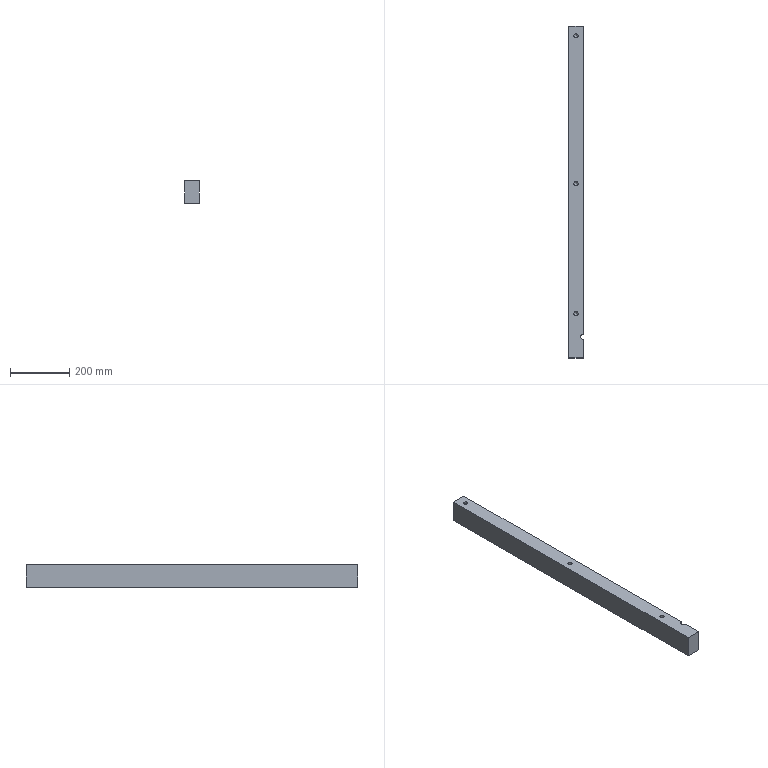Part | NX | features 3 2 | 1 solid | 20 faces | box 50 x 1123 x 75.5 mm | volume 4220069 mm3 | plane 7 | cylinder 7 | cone 6 | commonest cylinder face diameters 14.1 x6 18 x1
STEP:
#1=CARTESIAN_POINT('',(2967.05,-82.5,256.5));
#2=VERTEX_POINT('',#1);
#3=CARTESIAN_POINT('',(2960.,-82.5,256.5));
#4=DIRECTION('',(0.,0.,-1.));
#5=DIRECTION('',(1.,0.,0.));
#6=AXIS2_PLACEMENT_3D('',#3,#4,#5);
#7=CIRCLE('',#6,7.05);
#8=EDGE_CURVE('',#2,#2,#7,.T.);
#9=ORIENTED_EDGE('',*,*,#8,.T.);
#10=EDGE_LOOP('',(#9));
#11=FACE_BOUND('',#10,.T.);
#12=CARTESIAN_POINT('',(2985.,-672.5,256.5));
#13=VERTEX_POINT('',#12);
#14=CARTESIAN_POINT('',(2985.,-609.5,256.5));
#15=VERTEX_POINT('',#14);
#16=CARTESIAN_POINT('',(2985.,193.,256.5));
#17=DIRECTION('',(0.,1.,0.));
#18=VECTOR('',#17,1000.);
#19=LINE('',#16,#18);
#20=EDGE_CURVE('',#13,#15,#19,.T.);
#21=ORIENTED_EDGE('',*,*,#20,.T.);
#22=CARTESIAN_POINT('',(2985.,-591.5,256.5));
#23=VERTEX_POINT('',#22);
#24=CARTESIAN_POINT('',(2985.,-600.5,256.5));
#25=DIRECTION('',(0.,0.,1.));
#26=DIRECTION('',(1.,0.,0.));
#27=AXIS2_PLACEMENT_3D('',#24,#25,#26);
#28=CIRCLE('',#27,9.);
#29=EDGE_CURVE('',#23,#15,#28,.T.);
#30=ORIENTED_EDGE('',*,*,#29,.F.);
#31=CARTESIAN_POINT('',(2985.,450.5,256.5));
#32=VERTEX_POINT('',#31);
#33=CARTESIAN_POINT('',(2985.,193.,256.5));
#34=DIRECTION('',(0.,1.,0.));
#35=VECTOR('',#34,1000.);
#36=LINE('',#33,#35);
#37=EDGE_CURVE('',#23,#32,#36,.T.);
#38=ORIENTED_EDGE('',*,*,#37,.T.);
#39=CARTESIAN_POINT('',(2935.,450.5,256.5));
#40=VERTEX_POINT('',#39);
#41=CARTESIAN_POINT('',(945.,450.5,256.5));
#42=DIRECTION('',(-1.,0.,0.));
#43=VECTOR('',#42,1000.);
#44=LINE('',#41,#43);
#45=EDGE_CURVE('',#32,#40,#44,.T.);
#46=ORIENTED_EDGE('',*,*,#45,.T.);
#47=CARTESIAN_POINT('',(2935.,-672.5,256.5));
#48=VERTEX_POINT('',#47);
#49=CARTESIAN_POINT('',(2935.,193.,256.5));
#50=DIRECTION('',(0.,-1.,0.));
#51=VECTOR('',#50,1000.);
#52=LINE('',#49,#51);
#53=EDGE_CURVE('',#40,#48,#52,.T.);
#54=ORIENTED_EDGE('',*,*,#53,.T.);
#55=CARTESIAN_POINT('',(945.,-672.5,256.5));
#56=DIRECTION('',(1.,0.,0.));
#57=VECTOR('',#56,1000.);
#58=LINE('',#55,#57);
#59=EDGE_CURVE('',#48,#13,#58,.T.);
#60=ORIENTED_EDGE('',*,*,#59,.T.);
#61=EDGE_LOOP('',(#21,#30,#38,#46,#54,#60));
#62=FACE_BOUND('',#61,.T.);
#63=CARTESIAN_POINT('',(2967.05,417.5,256.5));
#64=VERTEX_POINT('',#63);
#65=CARTESIAN_POINT('',(2960.,417.5,256.5));
#66=DIRECTION('',(0.,0.,-1.));
#67=DIRECTION('',(1.,0.,0.));
#68=AXIS2_PLACEMENT_3D('',#65,#66,#67);
#69=CIRCLE('',#68,7.05);
#70=EDGE_CURVE('',#64,#64,#69,.T.);
#71=ORIENTED_EDGE('',*,*,#70,.T.);
#72=EDGE_LOOP('',(#71));
#73=FACE_BOUND('',#72,.T.);
#74=CARTESIAN_POINT('',(2967.05,-522.5,256.5));
#75=VERTEX_POINT('',#74);
#76=CARTESIAN_POINT('',(2960.,-522.5,256.5));
#77=DIRECTION('',(0.,0.,-1.));
#78=DIRECTION('',(1.,0.,0.));
#79=AXIS2_PLACEMENT_3D('',#76,#77,#78);
#80=CIRCLE('',#79,7.05);
#81=EDGE_CURVE('',#75,#75,#80,.T.);
#82=ORIENTED_EDGE('',*,*,#81,.T.);
#83=EDGE_LOOP('',(#82));
#84=FACE_BOUND('',#83,.T.);
#85=CARTESIAN_POINT('',(945.,0.,256.5));
#86=DIRECTION('',(0.,0.,1.));
#87=DIRECTION('',(1.,0.,0.));
#88=AXIS2_PLACEMENT_3D('',#85,#86,#87);
#89=PLANE('',#88);
#90=ADVANCED_FACE('',(#11,#62,#73,#84),#89,.T.);
#91=CARTESIAN_POINT('',(2967.05,-522.5,181.));
#92=VERTEX_POINT('',#91);
#93=CARTESIAN_POINT('',(2960.,-522.5,181.));
#94=DIRECTION('',(0.,0.,1.));
#95=DIRECTION('',(1.,0.,0.));
#96=AXIS2_PLACEMENT_3D('',#93,#94,#95);
#97=CIRCLE('',#96,7.05);
#98=EDGE_CURVE('',#92,#92,#97,.T.);
#99=ORIENTED_EDGE('',*,*,#98,.T.);
#100=EDGE_LOOP('',(#99));
#101=FACE_BOUND('',#100,.T.);
#102=CARTESIAN_POINT('',(2985.,450.5,181.));
#103=VERTEX_POINT('',#102);
#104=CARTESIAN_POINT('',(2985.,-591.5,181.));
#105=VERTEX_POINT('',#104);
#106=CARTESIAN_POINT('',(2985.,193.,181.));
#107=DIRECTION('',(0.,-1.,0.));
#108=VECTOR('',#107,1000.);
#109=LINE('',#106,#108);
#110=EDGE_CURVE('',#103,#105,#109,.T.);
#111=ORIENTED_EDGE('',*,*,#110,.T.);
#112=CARTESIAN_POINT('',(2985.,-609.5,181.));
#113=VERTEX_POINT('',#112);
#114=CARTESIAN_POINT('',(2985.,-600.5,181.));
#115=DIRECTION('',(0.,0.,-1.));
#116=DIRECTION('',(-1.,0.,0.));
#117=AXIS2_PLACEMENT_3D('',#114,#115,#116);
#118=CIRCLE('',#117,9.);
#119=EDGE_CURVE('',#113,#105,#118,.T.);
#120=ORIENTED_EDGE('',*,*,#119,.F.);
#121=CARTESIAN_POINT('',(2985.,-672.5,181.));
#122=VERTEX_POINT('',#121);
#123=CARTESIAN_POINT('',(2985.,193.,181.));
#124=DIRECTION('',(0.,-1.,0.));
#125=VECTOR('',#124,1000.);
#126=LINE('',#123,#125);
#127=EDGE_CURVE('',#113,#122,#126,.T.);
#128=ORIENTED_EDGE('',*,*,#127,.T.);
#129=CARTESIAN_POINT('',(2935.,-672.5,181.));
#130=VERTEX_POINT('',#129);
#131=CARTESIAN_POINT('',(282.5,-672.5,181.));
#132=DIRECTION('',(1.,0.,0.));
#133=VECTOR('',#132,1000.);
#134=LINE('',#131,#133);
#135=EDGE_CURVE('',#130,#122,#134,.T.);
#136=ORIENTED_EDGE('',*,*,#135,.F.);
#137=CARTESIAN_POINT('',(2935.,450.5,181.));
#138=VERTEX_POINT('',#137);
#139=CARTESIAN_POINT('',(2935.,193.,181.));
#140=DIRECTION('',(0.,1.,0.));
#141=VECTOR('',#140,1000.);
#142=LINE('',#139,#141);
#143=EDGE_CURVE('',#130,#138,#142,.T.);
#144=ORIENTED_EDGE('',*,*,#143,.T.);
#145=CARTESIAN_POINT('',(1715.,450.5,181.));
#146=DIRECTION('',(1.,0.,0.));
#147=VECTOR('',#146,1000.);
#148=LINE('',#145,#147);
#149=EDGE_CURVE('',#138,#103,#148,.T.);
#150=ORIENTED_EDGE('',*,*,#149,.T.);
#151=EDGE_LOOP('',(#111,#120,#128,#136,#144,#150));
#152=FACE_BOUND('',#151,.T.);
#153=CARTESIAN_POINT('',(2967.05,-82.5,181.));
#154=VERTEX_POINT('',#153);
#155=CARTESIAN_POINT('',(2960.,-82.5,181.));
#156=DIRECTION('',(0.,0.,1.));
#157=DIRECTION('',(1.,0.,0.));
#158=AXIS2_PLACEMENT_3D('',#155,#156,#157);
#159=CIRCLE('',#158,7.05);
#160=EDGE_CURVE('',#154,#154,#159,.T.);
#161=ORIENTED_EDGE('',*,*,#160,.T.);
#162=EDGE_LOOP('',(#161));
#163=FACE_BOUND('',#162,.T.);
#164=CARTESIAN_POINT('',(2967.05,417.5,181.));
#165=VERTEX_POINT('',#164);
#166=CARTESIAN_POINT('',(2960.,417.5,181.));
#167=DIRECTION('',(0.,0.,1.));
#168=DIRECTION('',(1.,0.,0.));
#169=AXIS2_PLACEMENT_3D('',#166,#167,#168);
#170=CIRCLE('',#169,7.05);
#171=EDGE_CURVE('',#165,#165,#170,.T.);
#172=ORIENTED_EDGE('',*,*,#171,.T.);
#173=EDGE_LOOP('',(#172));
#174=FACE_BOUND('',#173,.T.);
#175=CARTESIAN_POINT('',(1715.,193.,181.));
#176=DIRECTION('',(0.,0.,-1.));
#177=DIRECTION('',(1.,0.,0.));
#178=AXIS2_PLACEMENT_3D('',#175,#176,#177);
#179=PLANE('',#178);
#180=ADVANCED_FACE('',(#101,#152,#163,#174),#179,.T.);
#181=ORIENTED_EDGE('',*,*,#37,.F.);
#182=CARTESIAN_POINT('',(2985.,-591.5,-306.5));
#183=DIRECTION('',(0.,0.,-1.));
#184=VECTOR('',#183,1000.);
#185=LINE('',#182,#184);
#186=EDGE_CURVE('',#23,#105,#185,.T.);
#187=ORIENTED_EDGE('',*,*,#186,.T.);
#188=ORIENTED_EDGE('',*,*,#110,.F.);
#189=CARTESIAN_POINT('',(2985.,450.5,-1.5));
#190=DIRECTION('',(0.,0.,1.));
#191=VECTOR('',#190,1000.);
#192=LINE('',#189,#191);
#193=EDGE_CURVE('',#103,#32,#192,.T.);
#194=ORIENTED_EDGE('',*,*,#193,.T.);
#195=EDGE_LOOP('',(#181,#187,#188,#194));
#196=FACE_BOUND('',#195,.T.);
#197=CARTESIAN_POINT('',(2985.,193.,-1.5));
#198=DIRECTION('',(1.,0.,0.));
#199=DIRECTION('',(0.,0.,-1.));
#200=AXIS2_PLACEMENT_3D('',#197,#198,#199);
#201=PLANE('',#200);
#202=ADVANCED_FACE('',(#196),#201,.T.);
#203=ORIENTED_EDGE('',*,*,#127,.F.);
#204=CARTESIAN_POINT('',(2985.,-609.5,-306.5));
#205=DIRECTION('',(0.,0.,1.));
#206=VECTOR('',#205,1000.);
#207=LINE('',#204,#206);
#208=EDGE_CURVE('',#113,#15,#207,.T.);
#209=ORIENTED_EDGE('',*,*,#208,.T.);
#210=ORIENTED_EDGE('',*,*,#20,.F.);
#211=CARTESIAN_POINT('',(2985.,-672.5,-103.));
#212=DIRECTION('',(0.,0.,1.));
#213=VECTOR('',#212,1000.);
#214=LINE('',#211,#213);
#215=EDGE_CURVE('',#122,#13,#214,.T.);
#216=ORIENTED_EDGE('',*,*,#215,.F.);
#217=EDGE_LOOP('',(#203,#209,#210,#216));
#218=FACE_BOUND('',#217,.T.);
#219=CARTESIAN_POINT('',(2985.,193.,-1.5));
#220=DIRECTION('',(1.,0.,0.));
#221=DIRECTION('',(0.,0.,-1.));
#222=AXIS2_PLACEMENT_3D('',#219,#220,#221);
#223=PLANE('',#222);
#224=ADVANCED_FACE('',(#218),#223,.T.);
#225=ORIENTED_EDGE('',*,*,#45,.F.);
#226=ORIENTED_EDGE('',*,*,#193,.F.);
#227=ORIENTED_EDGE('',*,*,#149,.F.);
#228=CARTESIAN_POINT('',(2935.,450.5,-1.5));
#229=DIRECTION('',(0.,0.,-1.));
#230=VECTOR('',#229,1000.);
#231=LINE('',#228,#230);
#232=EDGE_CURVE('',#40,#138,#231,.T.);
#233=ORIENTED_EDGE('',*,*,#232,.F.);
#234=EDGE_LOOP('',(#225,#226,#227,#233));
#235=FACE_BOUND('',#234,.T.);
#236=CARTESIAN_POINT('',(2813.,450.5,179.));
#237=DIRECTION('',(0.,1.,0.));
#238=DIRECTION('',(0.,0.,-1.));
#239=AXIS2_PLACEMENT_3D('',#236,#237,#238);
#240=PLANE('',#239);
#241=ADVANCED_FACE('',(#235),#240,.T.);
#242=ORIENTED_EDGE('',*,*,#53,.F.);
#243=ORIENTED_EDGE('',*,*,#232,.T.);
#244=ORIENTED_EDGE('',*,*,#143,.F.);
#245=CARTESIAN_POINT('',(2935.,-672.5,-103.));
#246=DIRECTION('',(0.,0.,-1.));
#247=VECTOR('',#246,1000.);
#248=LINE('',#245,#247);
#249=EDGE_CURVE('',#48,#130,#248,.T.);
#250=ORIENTED_EDGE('',*,*,#249,.F.);
#251=EDGE_LOOP('',(#242,#243,#244,#250));
#252=FACE_BOUND('',#251,.T.);
#253=CARTESIAN_POINT('',(2935.,193.,-1.5));
#254=DIRECTION('',(-1.,0.,0.));
#255=DIRECTION('',(0.,0.,1.));
#256=AXIS2_PLACEMENT_3D('',#253,#254,#255);
#257=PLANE('',#256);
#258=ADVANCED_FACE('',(#252),#257,.T.);
#259=ORIENTED_EDGE('',*,*,#249,.T.);
#260=ORIENTED_EDGE('',*,*,#135,.T.);
#261=ORIENTED_EDGE('',*,*,#215,.T.);
#262=ORIENTED_EDGE('',*,*,#59,.F.);
#263=EDGE_LOOP('',(#259,#260,#261,#262));
#264=FACE_BOUND('',#263,.T.);
#265=CARTESIAN_POINT('',(282.5,-672.5,-103.));
#266=DIRECTION('',(0.,1.,0.));
#267=DIRECTION('',(1.,0.,0.));
#268=AXIS2_PLACEMENT_3D('',#265,#266,#267);
#269=PLANE('',#268);
#270=ADVANCED_FACE('',(#264),#269,.F.);
#271=ORIENTED_EDGE('',*,*,#29,.T.);
#272=ORIENTED_EDGE('',*,*,#208,.F.);
#273=ORIENTED_EDGE('',*,*,#119,.T.);
#274=ORIENTED_EDGE('',*,*,#186,.F.);
#275=EDGE_LOOP('',(#271,#272,#273,#274));
#276=FACE_BOUND('',#275,.T.);
#277=CARTESIAN_POINT('',(2985.,-600.5,-306.5));
#278=DIRECTION('',(0.,0.,1.));
#279=DIRECTION('',(-1.,0.,0.));
#280=AXIS2_PLACEMENT_3D('',#277,#278,#279);
#281=CYLINDRICAL_SURFACE('',#280,9.);
#282=ADVANCED_FACE('',(#276),#281,.F.);
#283=CARTESIAN_POINT('',(2967.05,-82.5,188.95));
#284=VERTEX_POINT('',#283);
#285=CARTESIAN_POINT('',(2960.,-82.5,188.95));
#286=DIRECTION('',(0.,0.,1.));
#287=DIRECTION('',(1.,0.,0.));
#288=AXIS2_PLACEMENT_3D('',#285,#286,#287);
#289=CIRCLE('',#288,7.05);
#290=EDGE_CURVE('',#284,#284,#289,.T.);
#291=ORIENTED_EDGE('',*,*,#290,.T.);
#292=EDGE_LOOP('',(#291));
#293=FACE_BOUND('',#292,.T.);
#294=ORIENTED_EDGE('',*,*,#160,.F.);
#295=EDGE_LOOP('',(#294));
#296=FACE_BOUND('',#295,.T.);
#297=CARTESIAN_POINT('',(2960.,-82.5,181.));
#298=DIRECTION('',(0.,0.,1.));
#299=DIRECTION('',(-1.,0.,0.));
#300=AXIS2_PLACEMENT_3D('',#297,#298,#299);
#301=CYLINDRICAL_SURFACE('',#300,7.05);
#302=ADVANCED_FACE('',(#293,#296),#301,.F.);
#303=CARTESIAN_POINT('',(2960.,-82.5,196.));
#304=VERTEX_POINT('',#303);
#305=VERTEX_LOOP('',#304);
#306=FACE_BOUND('',#305,.T.);
#307=ORIENTED_EDGE('',*,*,#290,.F.);
#308=EDGE_LOOP('',(#307));
#309=FACE_BOUND('',#308,.T.);
#310=CARTESIAN_POINT('',(2960.,-82.5,188.95));
#311=DIRECTION('',(0.,0.,-1.));
#312=DIRECTION('',(1.,0.,0.));
#313=AXIS2_PLACEMENT_3D('',#310,#311,#312);
#314=CONICAL_SURFACE('',#313,7.05,0.7854);
#315=ADVANCED_FACE('',(#306,#309),#314,.F.);
#316=CARTESIAN_POINT('',(2967.05,-522.5,188.95));
#317=VERTEX_POINT('',#316);
#318=CARTESIAN_POINT('',(2960.,-522.5,188.95));
#319=DIRECTION('',(0.,0.,1.));
#320=DIRECTION('',(1.,0.,0.));
#321=AXIS2_PLACEMENT_3D('',#318,#319,#320);
#322=CIRCLE('',#321,7.05);
#323=EDGE_CURVE('',#317,#317,#322,.T.);
#324=ORIENTED_EDGE('',*,*,#323,.T.);
#325=EDGE_LOOP('',(#324));
#326=FACE_BOUND('',#325,.T.);
#327=ORIENTED_EDGE('',*,*,#98,.F.);
#328=EDGE_LOOP('',(#327));
#329=FACE_BOUND('',#328,.T.);
#330=CARTESIAN_POINT('',(2960.,-522.5,181.));
#331=DIRECTION('',(0.,0.,1.));
#332=DIRECTION('',(-1.,0.,0.));
#333=AXIS2_PLACEMENT_3D('',#330,#331,#332);
#334=CYLINDRICAL_SURFACE('',#333,7.05);
#335=ADVANCED_FACE('',(#326,#329),#334,.F.);
#336=CARTESIAN_POINT('',(2960.,-522.5,196.));
#337=VERTEX_POINT('',#336);
#338=VERTEX_LOOP('',#337);
#339=FACE_BOUND('',#338,.T.);
#340=ORIENTED_EDGE('',*,*,#323,.F.);
#341=EDGE_LOOP('',(#340));
#342=FACE_BOUND('',#341,.T.);
#343=CARTESIAN_POINT('',(2960.,-522.5,188.95));
#344=DIRECTION('',(0.,0.,-1.));
#345=DIRECTION('',(1.,0.,0.));
#346=AXIS2_PLACEMENT_3D('',#343,#344,#345);
#347=CONICAL_SURFACE('',#346,7.05,0.7854);
#348=ADVANCED_FACE('',(#339,#342),#347,.F.);
#349=CARTESIAN_POINT('',(2967.05,417.5,188.95));
#350=VERTEX_POINT('',#349);
#351=CARTESIAN_POINT('',(2960.,417.5,188.95));
#352=DIRECTION('',(0.,0.,1.));
#353=DIRECTION('',(1.,0.,0.));
#354=AXIS2_PLACEMENT_3D('',#351,#352,#353);
#355=CIRCLE('',#354,7.05);
#356=EDGE_CURVE('',#350,#350,#355,.T.);
#357=ORIENTED_EDGE('',*,*,#356,.T.);
#358=EDGE_LOOP('',(#357));
#359=FACE_BOUND('',#358,.T.);
#360=ORIENTED_EDGE('',*,*,#171,.F.);
#361=EDGE_LOOP('',(#360));
#362=FACE_BOUND('',#361,.T.);
#363=CARTESIAN_POINT('',(2960.,417.5,181.));
#364=DIRECTION('',(0.,0.,1.));
#365=DIRECTION('',(-1.,0.,0.));
#366=AXIS2_PLACEMENT_3D('',#363,#364,#365);
#367=CYLINDRICAL_SURFACE('',#366,7.05);
#368=ADVANCED_FACE('',(#359,#362),#367,.F.);
#369=CARTESIAN_POINT('',(2960.,417.5,196.));
#370=VERTEX_POINT('',#369);
#371=VERTEX_LOOP('',#370);
#372=FACE_BOUND('',#371,.T.);
#373=ORIENTED_EDGE('',*,*,#356,.F.);
#374=EDGE_LOOP('',(#373));
#375=FACE_BOUND('',#374,.T.);
#376=CARTESIAN_POINT('',(2960.,417.5,188.95));
#377=DIRECTION('',(0.,0.,-1.));
#378=DIRECTION('',(1.,0.,0.));
#379=AXIS2_PLACEMENT_3D('',#376,#377,#378);
#380=CONICAL_SURFACE('',#379,7.05,0.7854);
#381=ADVANCED_FACE('',(#372,#375),#380,.F.);
#382=CARTESIAN_POINT('',(2952.95,417.5,248.55));
#383=VERTEX_POINT('',#382);
#384=CARTESIAN_POINT('',(2960.,417.5,248.55));
#385=DIRECTION('',(0.,0.,-1.));
#386=DIRECTION('',(-1.,0.,0.));
#387=AXIS2_PLACEMENT_3D('',#384,#385,#386);
#388=CIRCLE('',#387,7.05);
#389=EDGE_CURVE('',#383,#383,#388,.T.);
#390=ORIENTED_EDGE('',*,*,#389,.T.);
#391=EDGE_LOOP('',(#390));
#392=FACE_BOUND('',#391,.T.);
#393=ORIENTED_EDGE('',*,*,#70,.F.);
#394=EDGE_LOOP('',(#393));
#395=FACE_BOUND('',#394,.T.);
#396=CARTESIAN_POINT('',(2960.,417.5,256.5));
#397=DIRECTION('',(0.,0.,-1.));
#398=DIRECTION('',(-1.,0.,0.));
#399=AXIS2_PLACEMENT_3D('',#396,#397,#398);
#400=CYLINDRICAL_SURFACE('',#399,7.05);
#401=ADVANCED_FACE('',(#392,#395),#400,.F.);
#402=CARTESIAN_POINT('',(2960.,417.5,241.5));
#403=VERTEX_POINT('',#402);
#404=VERTEX_LOOP('',#403);
#405=FACE_BOUND('',#404,.T.);
#406=ORIENTED_EDGE('',*,*,#389,.F.);
#407=EDGE_LOOP('',(#406));
#408=FACE_BOUND('',#407,.T.);
#409=CARTESIAN_POINT('',(2960.,417.5,248.55));
#410=DIRECTION('',(0.,0.,1.));
#411=DIRECTION('',(-1.,0.,0.));
#412=AXIS2_PLACEMENT_3D('',#409,#410,#411);
#413=CONICAL_SURFACE('',#412,7.05,0.7854);
#414=ADVANCED_FACE('',(#405,#408),#413,.F.);
#415=CARTESIAN_POINT('',(2952.95,-82.5,248.55));
#416=VERTEX_POINT('',#415);
#417=CARTESIAN_POINT('',(2960.,-82.5,248.55));
#418=DIRECTION('',(0.,0.,-1.));
#419=DIRECTION('',(-1.,0.,0.));
#420=AXIS2_PLACEMENT_3D('',#417,#418,#419);
#421=CIRCLE('',#420,7.05);
#422=EDGE_CURVE('',#416,#416,#421,.T.);
#423=ORIENTED_EDGE('',*,*,#422,.T.);
#424=EDGE_LOOP('',(#423));
#425=FACE_BOUND('',#424,.T.);
#426=ORIENTED_EDGE('',*,*,#8,.F.);
#427=EDGE_LOOP('',(#426));
#428=FACE_BOUND('',#427,.T.);
#429=CARTESIAN_POINT('',(2960.,-82.5,256.5));
#430=DIRECTION('',(0.,0.,-1.));
#431=DIRECTION('',(-1.,0.,0.));
#432=AXIS2_PLACEMENT_3D('',#429,#430,#431);
#433=CYLINDRICAL_SURFACE('',#432,7.05);
#434=ADVANCED_FACE('',(#425,#428),#433,.F.);
#435=CARTESIAN_POINT('',(2960.,-82.5,241.5));
#436=VERTEX_POINT('',#435);
#437=VERTEX_LOOP('',#436);
#438=FACE_BOUND('',#437,.T.);
#439=ORIENTED_EDGE('',*,*,#422,.F.);
#440=EDGE_LOOP('',(#439));
#441=FACE_BOUND('',#440,.T.);
#442=CARTESIAN_POINT('',(2960.,-82.5,248.55));
#443=DIRECTION('',(0.,0.,1.));
#444=DIRECTION('',(-1.,0.,0.));
#445=AXIS2_PLACEMENT_3D('',#442,#443,#444);
#446=CONICAL_SURFACE('',#445,7.05,0.7854);
#447=ADVANCED_FACE('',(#438,#441),#446,.F.);
#448=CARTESIAN_POINT('',(2952.95,-522.5,248.55));
#449=VERTEX_POINT('',#448);
#450=CARTESIAN_POINT('',(2960.,-522.5,248.55));
#451=DIRECTION('',(0.,0.,-1.));
#452=DIRECTION('',(-1.,0.,0.));
#453=AXIS2_PLACEMENT_3D('',#450,#451,#452);
#454=CIRCLE('',#453,7.05);
#455=EDGE_CURVE('',#449,#449,#454,.T.);
#456=ORIENTED_EDGE('',*,*,#455,.T.);
#457=EDGE_LOOP('',(#456));
#458=FACE_BOUND('',#457,.T.);
#459=ORIENTED_EDGE('',*,*,#81,.F.);
#460=EDGE_LOOP('',(#459));
#461=FACE_BOUND('',#460,.T.);
#462=CARTESIAN_POINT('',(2960.,-522.5,256.5));
#463=DIRECTION('',(0.,0.,-1.));
#464=DIRECTION('',(-1.,0.,0.));
#465=AXIS2_PLACEMENT_3D('',#462,#463,#464);
#466=CYLINDRICAL_SURFACE('',#465,7.05);
#467=ADVANCED_FACE('',(#458,#461),#466,.F.);
#468=CARTESIAN_POINT('',(2960.,-522.5,241.5));
#469=VERTEX_POINT('',#468);
#470=VERTEX_LOOP('',#469);
#471=FACE_BOUND('',#470,.T.);
#472=ORIENTED_EDGE('',*,*,#455,.F.);
#473=EDGE_LOOP('',(#472));
#474=FACE_BOUND('',#473,.T.);
#475=CARTESIAN_POINT('',(2960.,-522.5,248.55));
#476=DIRECTION('',(0.,0.,1.));
#477=DIRECTION('',(-1.,0.,0.));
#478=AXIS2_PLACEMENT_3D('',#475,#476,#477);
#479=CONICAL_SURFACE('',#478,7.05,0.7854);
#480=ADVANCED_FACE('',(#471,#474),#479,.F.);
#481=CLOSED_SHELL('',(#90,#180,#202,#224,#241,#258,#270,#282,#302,#315,#335,#348,#368,#381,#401,#414,#434,#447,#467,#480));
#482=MANIFOLD_SOLID_BREP('',#481);
#483=(LENGTH_UNIT()NAMED_UNIT(*)SI_UNIT(.MILLI.,.METRE.));
#484=UNCERTAINTY_MEASURE_WITH_UNIT(LENGTH_MEASURE(0.00001),#483,'','');
#485=(NAMED_UNIT(*)PLANE_ANGLE_UNIT()SI_UNIT($,.RADIAN.));
#486=(NAMED_UNIT(*)SI_UNIT($,.STERADIAN.)SOLID_ANGLE_UNIT());
#487=(GEOMETRIC_REPRESENTATION_CONTEXT(3)GLOBAL_UNCERTAINTY_ASSIGNED_CONTEXT((#484))GLOBAL_UNIT_ASSIGNED_CONTEXT((#483,#485,#486))REPRESENTATION_CONTEXT('',''));
#488=ADVANCED_BREP_SHAPE_REPRESENTATION('',(#482),#487);